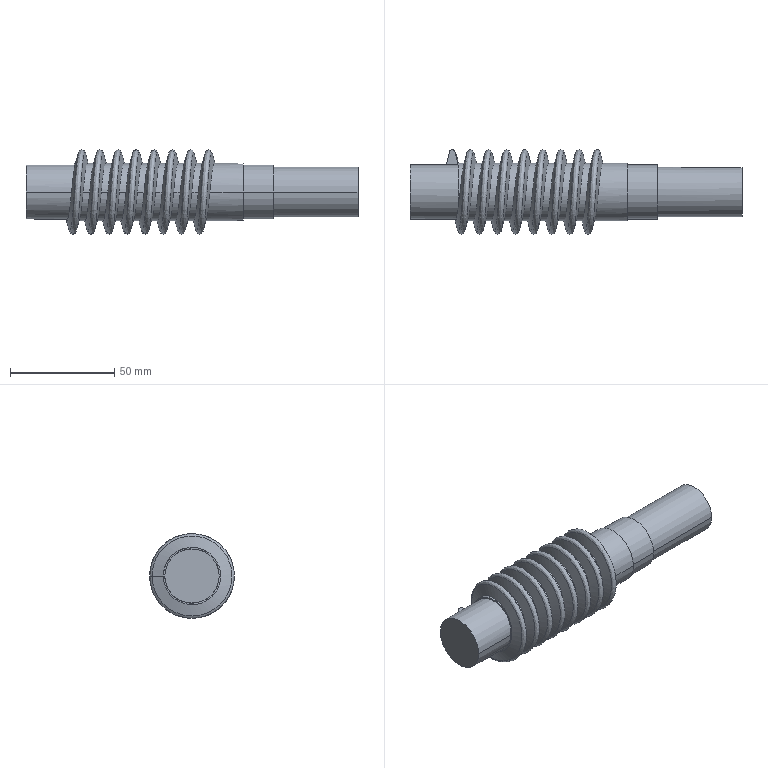Part | SolidWorks | features Helix 2, Sweep 2, ICE 1, Revolution 1, Scale 1 | 1 solid | 43 faces | box 158.95 x 40.46 x 40.46 mm | volume 106297 mm3 | cylinder 24 | plane 11 | spline 8 | commonest cylinder face diameters 27.455 x17 26.01 x5 23.843 x2